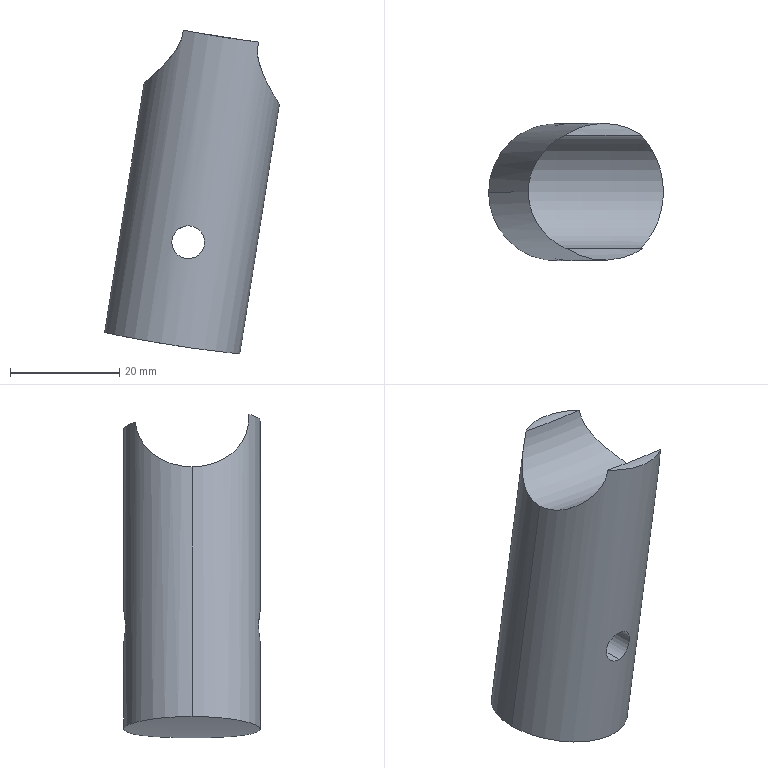Part | SolidWorks | features HoleWzd 2, RefAxis 2, 3DProfileFeature 1, CirPattern 1, ICE 1, Revolution 1 | 1 solid | 8 faces | box 31.917 x 25 x 59.146 mm | volume 23195 mm3 | cylinder 7 | torus 1 | commonest cylinder face diameters 6 x2 25 x2 352 x1 355 x1 466 x1
STEP:
#1=CARTESIAN_POINT('',(-33.477,15.509,-214.365));
#2=VERTEX_POINT('',#1);
#3=CARTESIAN_POINT('',(-33.477,15.509,-208.365));
#4=VERTEX_POINT('',#3);
#5=CARTESIAN_POINT('',(-33.477,15.509,-214.365));
#6=CARTESIAN_POINT('',(-33.869,15.494,-214.365));
#7=CARTESIAN_POINT('',(-34.266,15.498,-214.286));
#8=CARTESIAN_POINT('',(-34.808,15.531,-214.061));
#9=CARTESIAN_POINT('',(-34.984,15.546,-213.967));
#10=CARTESIAN_POINT('',(-35.311,15.582,-213.748));
#11=CARTESIAN_POINT('',(-35.461,15.603,-213.624));
#12=CARTESIAN_POINT('',(-35.738,15.648,-213.347));
#13=CARTESIAN_POINT('',(-35.864,15.672,-213.193));
#14=CARTESIAN_POINT('',(-36.08,15.719,-212.869));
#15=CARTESIAN_POINT('',(-36.172,15.743,-212.697));
#16=CARTESIAN_POINT('',(-36.324,15.786,-212.333));
#17=CARTESIAN_POINT('',(-36.381,15.805,-212.145));
#18=CARTESIAN_POINT('',(-36.457,15.836,-211.761));
#19=CARTESIAN_POINT('',(-36.477,15.849,-211.564));
#20=CARTESIAN_POINT('',(-36.477,15.864,-211.169));
#21=CARTESIAN_POINT('',(-36.458,15.867,-210.973));
#22=CARTESIAN_POINT('',(-36.381,15.863,-210.588));
#23=CARTESIAN_POINT('',(-36.323,15.856,-210.396));
#24=CARTESIAN_POINT('',(-36.172,15.834,-210.034));
#25=CARTESIAN_POINT('',(-36.08,15.819,-209.861));
#26=CARTESIAN_POINT('',(-35.861,15.782,-209.533));
#27=CARTESIAN_POINT('',(-35.735,15.76,-209.381));
#28=CARTESIAN_POINT('',(-35.459,15.715,-209.105));
#29=CARTESIAN_POINT('',(-35.307,15.691,-208.98));
#30=CARTESIAN_POINT('',(-34.98,15.643,-208.762));
#31=CARTESIAN_POINT('',(-34.808,15.62,-208.67));
#32=CARTESIAN_POINT('',(-34.448,15.578,-208.52));
#33=CARTESIAN_POINT('',(-34.257,15.559,-208.462));
#34=CARTESIAN_POINT('',(-33.872,15.528,-208.385));
#35=CARTESIAN_POINT('',(-33.676,15.516,-208.365));
#36=CARTESIAN_POINT('',(-33.477,15.509,-208.365));
#37=B_SPLINE_CURVE_WITH_KNOTS('',3,(#5,#6,#7,#8,#9,#10,#11,#12,#13,#14,#15,#16,#17,#18,#19,#20,#21,#22,#23,#24,#25,#26,#27,#28,#29,#30,#31,#32,#33,#34,#35,#36),.UNSPECIFIED.,.F.,.F.,(4,2,2,2,2,2,2,2,2,2,2,2,2,2,2,4),(0.009415,0.01059,0.01118,0.01177,0.01236,0.01294,0.01353,0.01412,0.01471,0.0153,0.01589,0.01647,0.01706,0.01765,0.01824,0.01883),.UNSPECIFIED.);
#38=EDGE_CURVE('',#2,#4,#37,.T.);
#39=ORIENTED_EDGE('',*,*,#38,.F.);
#40=CARTESIAN_POINT('',(-33.477,40.491,-214.365));
#41=VERTEX_POINT('',#40);
#42=CARTESIAN_POINT('',(-33.477,40.5,-214.365));
#43=DIRECTION('',(0.,1.,0.));
#44=VECTOR('',#43,1000.);
#45=LINE('',#42,#44);
#46=EDGE_CURVE('',#2,#41,#45,.T.);
#47=ORIENTED_EDGE('',*,*,#46,.T.);
#48=CARTESIAN_POINT('',(-33.477,40.491,-208.365));
#49=VERTEX_POINT('',#48);
#50=CARTESIAN_POINT('',(-33.477,40.491,-208.365));
#51=CARTESIAN_POINT('',(-33.676,40.484,-208.365));
#52=CARTESIAN_POINT('',(-33.871,40.472,-208.385));
#53=CARTESIAN_POINT('',(-34.255,40.441,-208.461));
#54=CARTESIAN_POINT('',(-34.445,40.422,-208.519));
#55=CARTESIAN_POINT('',(-34.808,40.38,-208.669));
#56=CARTESIAN_POINT('',(-34.979,40.357,-208.761));
#57=CARTESIAN_POINT('',(-35.305,40.31,-208.978));
#58=CARTESIAN_POINT('',(-35.458,40.285,-209.104));
#59=CARTESIAN_POINT('',(-35.735,40.24,-209.38));
#60=CARTESIAN_POINT('',(-35.859,40.218,-209.531));
#61=CARTESIAN_POINT('',(-36.078,40.181,-209.858));
#62=CARTESIAN_POINT('',(-36.172,40.166,-210.033));
#63=CARTESIAN_POINT('',(-36.322,40.144,-210.394));
#64=CARTESIAN_POINT('',(-36.38,40.137,-210.584));
#65=CARTESIAN_POINT('',(-36.458,40.133,-210.972));
#66=CARTESIAN_POINT('',(-36.477,40.136,-211.168));
#67=CARTESIAN_POINT('',(-36.477,40.151,-211.56));
#68=CARTESIAN_POINT('',(-36.457,40.163,-211.76));
#69=CARTESIAN_POINT('',(-36.381,40.195,-212.144));
#70=CARTESIAN_POINT('',(-36.324,40.214,-212.331));
#71=CARTESIAN_POINT('',(-36.174,40.257,-212.695));
#72=CARTESIAN_POINT('',(-36.08,40.281,-212.869));
#73=CARTESIAN_POINT('',(-35.864,40.328,-213.193));
#74=CARTESIAN_POINT('',(-35.74,40.352,-213.345));
#75=CARTESIAN_POINT('',(-35.461,40.397,-213.624));
#76=CARTESIAN_POINT('',(-35.31,40.418,-213.748));
#77=CARTESIAN_POINT('',(-34.986,40.454,-213.966));
#78=CARTESIAN_POINT('',(-34.81,40.469,-214.06));
#79=CARTESIAN_POINT('',(-34.446,40.491,-214.211));
#80=CARTESIAN_POINT('',(-34.259,40.497,-214.268));
#81=CARTESIAN_POINT('',(-33.873,40.501,-214.346));
#82=CARTESIAN_POINT('',(-33.673,40.498,-214.365));
#83=CARTESIAN_POINT('',(-33.477,40.491,-214.365));
#84=B_SPLINE_CURVE_WITH_KNOTS('',3,(#50,#51,#52,#53,#54,#55,#56,#57,#58,#59,#60,#61,#62,#63,#64,#65,#66,#67,#68,#69,#70,#71,#72,#73,#74,#75,#76,#77,#78,#79,#80,#81,#82,#83),.UNSPECIFIED.,.F.,.F.,(4,2,2,2,2,2,2,2,2,2,2,2,2,2,2,2,4),(0.,0.0005883,0.001177,0.001765,0.002353,0.002942,0.00353,0.004118,0.004707,0.005295,0.005883,0.006472,0.00706,0.007648,0.008236,0.008825,0.009413),.UNSPECIFIED.);
#85=EDGE_CURVE('',#49,#41,#84,.T.);
#86=ORIENTED_EDGE('',*,*,#85,.F.);
#87=CARTESIAN_POINT('',(-33.477,40.5,-208.365));
#88=DIRECTION('',(0.,1.,0.));
#89=VECTOR('',#88,1000.);
#90=LINE('',#87,#89);
#91=EDGE_CURVE('',#4,#49,#90,.T.);
#92=ORIENTED_EDGE('',*,*,#91,.F.);
#93=EDGE_LOOP('',(#39,#47,#86,#92));
#94=FACE_OUTER_BOUND('',#93,.T.);
#95=CARTESIAN_POINT('',(-33.477,40.5,-211.365));
#96=DIRECTION('',(0.,1.,0.));
#97=DIRECTION('',(0.,0.,1.));
#98=AXIS2_PLACEMENT_3D('',#95,#96,#97);
#99=CYLINDRICAL_SURFACE('',#98,3.);
#100=ADVANCED_FACE('',(#94),#99,.F.);
#101=ORIENTED_EDGE('',*,*,#85,.T.);
#102=CARTESIAN_POINT('',(-33.477,40.491,-214.365));
#103=CARTESIAN_POINT('',(-33.085,40.477,-214.365));
#104=CARTESIAN_POINT('',(-32.69,40.443,-214.286));
#105=CARTESIAN_POINT('',(-32.149,40.38,-214.062));
#106=CARTESIAN_POINT('',(-31.974,40.357,-213.969));
#107=CARTESIAN_POINT('',(-31.648,40.309,-213.751));
#108=CARTESIAN_POINT('',(-31.497,40.285,-213.628));
#109=CARTESIAN_POINT('',(-31.221,40.24,-213.352));
#110=CARTESIAN_POINT('',(-31.094,40.218,-213.198));
#111=CARTESIAN_POINT('',(-30.876,40.182,-212.873));
#112=CARTESIAN_POINT('',(-30.784,40.166,-212.701));
#113=CARTESIAN_POINT('',(-30.556,40.133,-212.154));
#114=CARTESIAN_POINT('',(-30.477,40.129,-211.762));
#115=CARTESIAN_POINT('',(-30.477,40.151,-211.169));
#116=CARTESIAN_POINT('',(-30.496,40.163,-210.974));
#117=CARTESIAN_POINT('',(-30.572,40.195,-210.589));
#118=CARTESIAN_POINT('',(-30.63,40.214,-210.398));
#119=CARTESIAN_POINT('',(-30.78,40.257,-210.037));
#120=CARTESIAN_POINT('',(-30.872,40.28,-209.865));
#121=CARTESIAN_POINT('',(-31.089,40.328,-209.538));
#122=CARTESIAN_POINT('',(-31.215,40.352,-209.385));
#123=CARTESIAN_POINT('',(-31.49,40.397,-209.11));
#124=CARTESIAN_POINT('',(-31.641,40.418,-208.984));
#125=CARTESIAN_POINT('',(-31.969,40.454,-208.764));
#126=CARTESIAN_POINT('',(-32.142,40.469,-208.672));
#127=CARTESIAN_POINT('',(-32.503,40.491,-208.521));
#128=CARTESIAN_POINT('',(-32.694,40.497,-208.462));
#129=CARTESIAN_POINT('',(-33.082,40.501,-208.385));
#130=CARTESIAN_POINT('',(-33.278,40.499,-208.365));
#131=CARTESIAN_POINT('',(-33.477,40.491,-208.365));
#132=B_SPLINE_CURVE_WITH_KNOTS('',3,(#102,#103,#104,#105,#106,#107,#108,#109,#110,#111,#112,#113,#114,#115,#116,#117,#118,#119,#120,#121,#122,#123,#124,#125,#126,#127,#128,#129,#130,#131),.UNSPECIFIED.,.F.,.F.,(4,2,2,2,2,2,2,2,2,2,2,2,2,2,4),(0.009413,0.01059,0.01118,0.01177,0.01235,0.01294,0.01412,0.01471,0.01529,0.01588,0.01647,0.01706,0.01765,0.01824,0.01882),.UNSPECIFIED.);
#133=EDGE_CURVE('',#41,#49,#132,.T.);
#134=ORIENTED_EDGE('',*,*,#133,.T.);
#135=EDGE_LOOP('',(#101,#134));
#136=FACE_BOUND('',#135,.T.);
#137=CARTESIAN_POINT('',(-48.743,28.,-227.845));
#138=VERTEX_POINT('',#137);
#139=CARTESIAN_POINT('',(-24.051,28.,-231.755));
#140=VERTEX_POINT('',#139);
#141=CARTESIAN_POINT('',(-48.743,28.,-227.845));
#142=CARTESIAN_POINT('',(-48.743,28.816,-227.845));
#143=CARTESIAN_POINT('',(-48.665,29.626,-227.861));
#144=CARTESIAN_POINT('',(-48.431,30.835,-227.911));
#145=CARTESIAN_POINT('',(-48.332,31.237,-227.932));
#146=CARTESIAN_POINT('',(-48.099,32.02,-227.981));
#147=CARTESIAN_POINT('',(-47.83,32.788,-228.038));
#148=CARTESIAN_POINT('',(-47.489,33.525,-228.109));
#149=CARTESIAN_POINT('',(-47.112,34.246,-228.187));
#150=CARTESIAN_POINT('',(-46.904,34.6,-228.23));
#151=CARTESIAN_POINT('',(-46.232,35.626,-228.368));
#152=CARTESIAN_POINT('',(-45.724,36.256,-228.47));
#153=CARTESIAN_POINT('',(-44.876,37.121,-228.638));
#154=CARTESIAN_POINT('',(-44.579,37.396,-228.696));
#155=CARTESIAN_POINT('',(-43.955,37.918,-228.817));
#156=CARTESIAN_POINT('',(-43.629,38.164,-228.879));
#157=CARTESIAN_POINT('',(-42.627,38.846,-229.069));
#158=CARTESIAN_POINT('',(-41.921,39.23,-229.199));
#159=CARTESIAN_POINT('',(-40.805,39.701,-229.399));
#160=CARTESIAN_POINT('',(-40.421,39.841,-229.467));
#161=CARTESIAN_POINT('',(-39.647,40.08,-229.602));
#162=CARTESIAN_POINT('',(-39.256,40.179,-229.67));
#163=CARTESIAN_POINT('',(-38.075,40.418,-229.869));
#164=CARTESIAN_POINT('',(-37.274,40.499,-230.001));
#165=CARTESIAN_POINT('',(-36.052,40.5,-230.194));
#166=CARTESIAN_POINT('',(-35.646,40.48,-230.258));
#167=CARTESIAN_POINT('',(-34.843,40.401,-230.38));
#168=CARTESIAN_POINT('',(-34.444,40.341,-230.44));
#169=CARTESIAN_POINT('',(-33.654,40.183,-230.557));
#170=CARTESIAN_POINT('',(-33.262,40.084,-230.614));
#171=CARTESIAN_POINT('',(-32.485,39.847,-230.725));
#172=CARTESIAN_POINT('',(-32.099,39.708,-230.779));
#173=CARTESIAN_POINT('',(-30.972,39.238,-230.934));
#174=CARTESIAN_POINT('',(-30.26,38.854,-231.028));
#175=CARTESIAN_POINT('',(-28.912,37.949,-231.2));
#176=CARTESIAN_POINT('',(-28.273,37.421,-231.279));
#177=CARTESIAN_POINT('',(-27.126,36.269,-231.416));
#178=CARTESIAN_POINT('',(-26.611,35.64,-231.476));
#179=CARTESIAN_POINT('',(-25.929,34.617,-231.553));
#180=CARTESIAN_POINT('',(-25.717,34.262,-231.576));
#181=CARTESIAN_POINT('',(-25.333,33.54,-231.619));
#182=CARTESIAN_POINT('',(-24.985,32.804,-231.657));
#183=CARTESIAN_POINT('',(-24.711,32.037,-231.686));
#184=CARTESIAN_POINT('',(-24.473,31.255,-231.711));
#185=CARTESIAN_POINT('',(-24.373,30.856,-231.722));
#186=CARTESIAN_POINT('',(-24.131,29.643,-231.747));
#187=CARTESIAN_POINT('',(-24.051,28.826,-231.755));
#188=CARTESIAN_POINT('',(-24.051,28.,-231.755));
#189=B_SPLINE_CURVE_WITH_KNOTS('',3,(#141,#142,#143,#144,#145,#146,#147,#148,#149,#150,#151,#152,#153,#154,#155,#156,#157,#158,#159,#160,#161,#162,#163,#164,#165,#166,#167,#168,#169,#170,#171,#172,#173,#174,#175,#176,#177,#178,#179,#180,#181,#182,#183,#184,#185,#186,#187,#188),.UNSPECIFIED.,.F.,.F.,(4,2,2,1,2,2,2,2,2,2,2,2,2,2,2,2,2,2,2,2,2,1,2,2,4),(0.03909,0.04153,0.04275,0.04397,0.04519,0.04641,0.04886,0.05008,0.0513,0.05374,0.05496,0.05618,0.05863,0.05985,0.06107,0.06229,0.06351,0.06595,0.0684,0.07084,0.07206,0.07328,0.0745,0.07572,0.07817),.UNSPECIFIED.);
#190=EDGE_CURVE('',#138,#140,#189,.T.);
#191=ORIENTED_EDGE('',*,*,#190,.F.);
#192=CARTESIAN_POINT('',(-41.518,28.,-182.23));
#193=VERTEX_POINT('',#192);
#194=CARTESIAN_POINT('',(-54.048,28.,-261.343));
#195=DIRECTION('',(0.1564,0.,0.9877));
#196=VECTOR('',#195,1000.);
#197=LINE('',#194,#196);
#198=EDGE_CURVE('',#138,#193,#197,.T.);
#199=ORIENTED_EDGE('',*,*,#198,.T.);
#200=CARTESIAN_POINT('',(-34.666,38.352,-174.082));
#201=VERTEX_POINT('',#200);
#202=CARTESIAN_POINT('',(-34.666,38.352,-174.082));
#203=CARTESIAN_POINT('',(-34.868,38.286,-174.737));
#204=CARTESIAN_POINT('',(-35.153,38.157,-175.336));
#205=CARTESIAN_POINT('',(-35.654,37.884,-176.181));
#206=CARTESIAN_POINT('',(-35.834,37.778,-176.454));
#207=CARTESIAN_POINT('',(-36.204,37.545,-176.976));
#208=CARTESIAN_POINT('',(-36.394,37.418,-177.225));
#209=CARTESIAN_POINT('',(-36.975,37.002,-177.944));
#210=CARTESIAN_POINT('',(-37.373,36.681,-178.387));
#211=CARTESIAN_POINT('',(-37.968,36.131,-179.01));
#212=CARTESIAN_POINT('',(-38.166,35.936,-179.21));
#213=CARTESIAN_POINT('',(-38.551,35.529,-179.591));
#214=CARTESIAN_POINT('',(-38.739,35.315,-179.772));
#215=CARTESIAN_POINT('',(-39.29,34.644,-180.293));
#216=CARTESIAN_POINT('',(-39.636,34.157,-180.608));
#217=CARTESIAN_POINT('',(-40.272,33.086,-181.172));
#218=CARTESIAN_POINT('',(-40.552,32.516,-181.414));
#219=CARTESIAN_POINT('',(-40.901,31.612,-181.712));
#220=CARTESIAN_POINT('',(-41.005,31.301,-181.801));
#221=CARTESIAN_POINT('',(-41.189,30.662,-181.955));
#222=CARTESIAN_POINT('',(-41.267,30.335,-182.021));
#223=CARTESIAN_POINT('',(-41.454,29.349,-182.177));
#224=CARTESIAN_POINT('',(-41.518,28.681,-182.23));
#225=CARTESIAN_POINT('',(-41.518,28.,-182.23));
#226=B_SPLINE_CURVE_WITH_KNOTS('',3,(#202,#203,#204,#205,#206,#207,#208,#209,#210,#211,#212,#213,#214,#215,#216,#217,#218,#219,#220,#221,#222,#223,#224,#225),.UNSPECIFIED.,.F.,.F.,(4,2,2,2,2,2,2,2,2,2,2,4),(0.000002056,0.00203,0.003044,0.004059,0.006087,0.007101,0.008115,0.01014,0.01217,0.01319,0.0142,0.01623),.UNSPECIFIED.);
#227=EDGE_CURVE('',#201,#193,#226,.T.);
#228=ORIENTED_EDGE('',*,*,#227,.F.);
#229=CARTESIAN_POINT('',(-20.825,38.352,-176.274));
#230=VERTEX_POINT('',#229);
#231=CARTESIAN_POINT('',(-20.825,38.352,-176.274));
#232=CARTESIAN_POINT('',(-21.854,39.052,-176.153));
#233=CARTESIAN_POINT('',(-22.958,39.584,-176.013));
#234=CARTESIAN_POINT('',(-24.429,40.04,-175.811));
#235=CARTESIAN_POINT('',(-24.729,40.121,-175.769));
#236=CARTESIAN_POINT('',(-25.33,40.258,-175.684));
#237=CARTESIAN_POINT('',(-25.631,40.316,-175.64));
#238=CARTESIAN_POINT('',(-26.537,40.453,-175.506));
#239=CARTESIAN_POINT('',(-27.145,40.499,-175.413));
#240=CARTESIAN_POINT('',(-28.367,40.501,-175.22));
#241=CARTESIAN_POINT('',(-28.986,40.454,-175.118));
#242=CARTESIAN_POINT('',(-30.194,40.271,-174.914));
#243=CARTESIAN_POINT('',(-30.787,40.135,-174.811));
#244=CARTESIAN_POINT('',(-31.658,39.865,-174.654));
#245=CARTESIAN_POINT('',(-31.946,39.764,-174.602));
#246=CARTESIAN_POINT('',(-32.515,39.539,-174.497));
#247=CARTESIAN_POINT('',(-32.797,39.414,-174.444));
#248=CARTESIAN_POINT('',(-33.627,39.011,-174.286));
#249=CARTESIAN_POINT('',(-34.158,38.702,-174.183));
#250=CARTESIAN_POINT('',(-34.666,38.352,-174.082));
#251=B_SPLINE_CURVE_WITH_KNOTS('',3,(#231,#232,#233,#234,#235,#236,#237,#238,#239,#240,#241,#242,#243,#244,#245,#246,#247,#248,#249,#250),.UNSPECIFIED.,.F.,.F.,(4,2,2,2,2,2,2,2,2,4),(0.,0.003698,0.004623,0.005547,0.007396,0.009246,0.01109,0.01202,0.01294,0.01479),.UNSPECIFIED.);
#252=EDGE_CURVE('',#230,#201,#251,.T.);
#253=ORIENTED_EDGE('',*,*,#252,.F.);
#254=CARTESIAN_POINT('',(-16.826,28.,-186.141));
#255=VERTEX_POINT('',#254);
#256=CARTESIAN_POINT('',(-16.826,28.,-186.141));
#257=CARTESIAN_POINT('',(-16.826,28.337,-186.141));
#258=CARTESIAN_POINT('',(-16.837,28.675,-186.124));
#259=CARTESIAN_POINT('',(-16.882,29.352,-186.053));
#260=CARTESIAN_POINT('',(-16.915,29.688,-186.));
#261=CARTESIAN_POINT('',(-17.045,30.673,-185.793));
#262=CARTESIAN_POINT('',(-17.172,31.308,-185.589));
#263=CARTESIAN_POINT('',(-17.496,32.525,-185.062));
#264=CARTESIAN_POINT('',(-17.687,33.092,-184.746));
#265=CARTESIAN_POINT('',(-18.007,33.888,-184.201));
#266=CARTESIAN_POINT('',(-18.119,34.145,-184.006));
#267=CARTESIAN_POINT('',(-18.351,34.638,-183.597));
#268=CARTESIAN_POINT('',(-18.47,34.873,-183.384));
#269=CARTESIAN_POINT('',(-18.834,35.545,-182.716));
#270=CARTESIAN_POINT('',(-19.085,35.95,-182.236));
#271=CARTESIAN_POINT('',(-19.458,36.5,-181.46));
#272=CARTESIAN_POINT('',(-19.581,36.672,-181.193));
#273=CARTESIAN_POINT('',(-19.819,36.993,-180.648));
#274=CARTESIAN_POINT('',(-19.934,37.142,-180.369));
#275=CARTESIAN_POINT('',(-20.262,37.556,-179.51));
#276=CARTESIAN_POINT('',(-20.458,37.788,-178.909));
#277=CARTESIAN_POINT('',(-20.675,38.063,-177.949));
#278=CARTESIAN_POINT('',(-20.734,38.142,-177.619));
#279=CARTESIAN_POINT('',(-20.811,38.27,-176.953));
#280=CARTESIAN_POINT('',(-20.83,38.319,-176.616));
#281=CARTESIAN_POINT('',(-20.825,38.352,-176.274));
#282=B_SPLINE_CURVE_WITH_KNOTS('',3,(#256,#257,#258,#259,#260,#261,#262,#263,#264,#265,#266,#267,#268,#269,#270,#271,#272,#273,#274,#275,#276,#277,#278,#279,#280,#281),.UNSPECIFIED.,.F.,.F.,(4,2,2,2,2,2,2,2,2,2,2,2,4),(0.05114,0.05215,0.05315,0.05516,0.05717,0.05818,0.05918,0.06119,0.0622,0.0632,0.06521,0.06622,0.06722),.UNSPECIFIED.);
#283=EDGE_CURVE('',#255,#230,#282,.T.);
#284=ORIENTED_EDGE('',*,*,#283,.F.);
#285=CARTESIAN_POINT('',(-29.356,28.,-265.254));
#286=DIRECTION('',(0.1564,0.,0.9877));
#287=VECTOR('',#286,1000.);
#288=LINE('',#285,#287);
#289=EDGE_CURVE('',#140,#255,#288,.T.);
#290=ORIENTED_EDGE('',*,*,#289,.F.);
#291=EDGE_LOOP('',(#191,#199,#228,#253,#284,#290));
#292=FACE_OUTER_BOUND('',#291,.T.);
#293=CARTESIAN_POINT('',(-41.702,28.,-263.299));
#294=DIRECTION('',(0.1564,0.,0.9877));
#295=DIRECTION('',(0.9877,0.,-0.1564));
#296=AXIS2_PLACEMENT_3D('',#293,#294,#295);
#297=CYLINDRICAL_SURFACE('',#296,12.5);
#298=ADVANCED_FACE('',(#136,#292),#297,.T.);
#299=CARTESIAN_POINT('',(-24.051,28.,-231.755));
#300=CARTESIAN_POINT('',(-24.051,27.174,-231.755));
#301=CARTESIAN_POINT('',(-24.131,26.362,-231.747));
#302=CARTESIAN_POINT('',(-24.369,25.163,-231.722));
#303=CARTESIAN_POINT('',(-24.467,24.767,-231.712));
#304=CARTESIAN_POINT('',(-24.704,23.982,-231.687));
#305=CARTESIAN_POINT('',(-24.843,23.591,-231.672));
#306=CARTESIAN_POINT('',(-25.312,22.456,-231.621));
#307=CARTESIAN_POINT('',(-25.694,21.738,-231.579));
#308=CARTESIAN_POINT('',(-26.371,20.719,-231.503));
#309=CARTESIAN_POINT('',(-26.615,20.388,-231.475));
#310=CARTESIAN_POINT('',(-27.135,19.751,-231.415));
#311=CARTESIAN_POINT('',(-27.408,19.448,-231.383));
#312=CARTESIAN_POINT('',(-28.268,18.583,-231.28));
#313=CARTESIAN_POINT('',(-28.893,18.066,-231.203));
#314=CARTESIAN_POINT('',(-29.91,17.38,-231.073));
#315=CARTESIAN_POINT('',(-30.262,17.168,-231.027));
#316=CARTESIAN_POINT('',(-30.977,16.782,-230.932));
#317=CARTESIAN_POINT('',(-31.708,16.434,-230.833));
#318=CARTESIAN_POINT('',(-32.468,16.159,-230.727));
#319=CARTESIAN_POINT('',(-33.243,15.921,-230.617));
#320=CARTESIAN_POINT('',(-33.64,15.82,-230.559));
#321=CARTESIAN_POINT('',(-34.837,15.58,-230.382));
#322=CARTESIAN_POINT('',(-35.639,15.5,-230.26));
#323=CARTESIAN_POINT('',(-36.848,15.5,-230.068));
#324=CARTESIAN_POINT('',(-37.251,15.52,-230.003));
#325=CARTESIAN_POINT('',(-38.06,15.6,-229.871));
#326=CARTESIAN_POINT('',(-38.463,15.661,-229.804));
#327=CARTESIAN_POINT('',(-39.649,15.9,-229.603));
#328=CARTESIAN_POINT('',(-40.416,16.136,-229.469));
#329=CARTESIAN_POINT('',(-41.534,16.606,-229.269));
#330=CARTESIAN_POINT('',(-41.903,16.783,-229.201));
#331=CARTESIAN_POINT('',(-42.615,17.17,-229.07));
#332=CARTESIAN_POINT('',(-42.959,17.38,-229.006));
#333=CARTESIAN_POINT('',(-43.958,18.059,-228.817));
#334=CARTESIAN_POINT('',(-44.578,18.576,-228.697));
#335=CARTESIAN_POINT('',(-45.724,19.743,-228.47));
#336=CARTESIAN_POINT('',(-46.232,20.375,-228.368));
#337=CARTESIAN_POINT('',(-46.898,21.39,-228.232));
#338=CARTESIAN_POINT('',(-47.104,21.74,-228.189));
#339=CARTESIAN_POINT('',(-47.483,22.463,-228.11));
#340=CARTESIAN_POINT('',(-47.657,22.838,-228.074));
#341=CARTESIAN_POINT('',(-48.118,23.974,-227.977));
#342=CARTESIAN_POINT('',(-48.35,24.753,-227.928));
#343=CARTESIAN_POINT('',(-48.585,25.955,-227.878));
#344=CARTESIAN_POINT('',(-48.644,26.362,-227.866));
#345=CARTESIAN_POINT('',(-48.723,27.183,-227.849));
#346=CARTESIAN_POINT('',(-48.743,27.592,-227.845));
#347=CARTESIAN_POINT('',(-48.743,28.,-227.845));
#348=B_SPLINE_CURVE_WITH_KNOTS('',3,(#299,#300,#301,#302,#303,#304,#305,#306,#307,#308,#309,#310,#311,#312,#313,#314,#315,#316,#317,#318,#319,#320,#321,#322,#323,#324,#325,#326,#327,#328,#329,#330,#331,#332,#333,#334,#335,#336,#337,#338,#339,#340,#341,#342,#343,#344,#345,#346,#347),.UNSPECIFIED.,.F.,.F.,(4,2,2,2,2,2,2,2,2,1,2,2,2,2,2,2,2,2,2,2,2,2,2,2,4),(0.,0.002443,0.003664,0.004886,0.007329,0.00855,0.009772,0.01221,0.01344,0.01466,0.01588,0.0171,0.01954,0.02077,0.02199,0.02443,0.02565,0.02687,0.02932,0.03176,0.03298,0.0342,0.03664,0.03787,0.03909),.UNSPECIFIED.);
#349=EDGE_CURVE('',#140,#138,#348,.T.);
#350=ORIENTED_EDGE('',*,*,#349,.T.);
#351=ORIENTED_EDGE('',*,*,#190,.T.);
#352=EDGE_LOOP('',(#350,#351));
#353=FACE_OUTER_BOUND('',#352,.T.);
#354=CARTESIAN_POINT('',(0.,33.104,0.));
#355=DIRECTION('',(0.,-1.,0.));
#356=DIRECTION('',(0.,0.,-1.));
#357=AXIS2_PLACEMENT_3D('',#354,#355,#356);
#358=CYLINDRICAL_SURFACE('',#357,233.);
#359=ADVANCED_FACE('',(#353),#358,.T.);
#360=ORIENTED_EDGE('',*,*,#198,.F.);
#361=ORIENTED_EDGE('',*,*,#349,.F.);
#362=ORIENTED_EDGE('',*,*,#289,.T.);
#363=CARTESIAN_POINT('',(-20.644,17.612,-174.785));
#364=VERTEX_POINT('',#363);
#365=CARTESIAN_POINT('',(-20.644,17.612,-174.785));
#366=CARTESIAN_POINT('',(-20.729,17.594,-175.149));
#367=CARTESIAN_POINT('',(-20.783,17.596,-175.516));
#368=CARTESIAN_POINT('',(-20.835,17.64,-176.251));
#369=CARTESIAN_POINT('',(-20.831,17.681,-176.623));
#370=CARTESIAN_POINT('',(-20.743,17.862,-177.727));
#371=CARTESIAN_POINT('',(-20.587,18.051,-178.425));
#372=CARTESIAN_POINT('',(-20.281,18.425,-179.433));
#373=CARTESIAN_POINT('',(-20.166,18.565,-179.76));
#374=CARTESIAN_POINT('',(-19.926,18.868,-180.391));
#375=CARTESIAN_POINT('',(-19.799,19.032,-180.696));
#376=CARTESIAN_POINT('',(-19.538,19.386,-181.287));
#377=CARTESIAN_POINT('',(-19.404,19.576,-181.574));
#378=CARTESIAN_POINT('',(-19.133,19.982,-182.13));
#379=CARTESIAN_POINT('',(-18.996,20.199,-182.4));
#380=CARTESIAN_POINT('',(-18.588,20.889,-183.178));
#381=CARTESIAN_POINT('',(-18.325,21.392,-183.648));
#382=CARTESIAN_POINT('',(-17.961,22.219,-184.279));
#383=CARTESIAN_POINT('',(-17.845,22.507,-184.477));
#384=CARTESIAN_POINT('',(-17.625,23.111,-184.847));
#385=CARTESIAN_POINT('',(-17.52,23.428,-185.02));
#386=CARTESIAN_POINT('',(-17.238,24.401,-185.484));
#387=CARTESIAN_POINT('',(-17.087,25.083,-185.725));
#388=CARTESIAN_POINT('',(-16.932,26.162,-185.974));
#389=CARTESIAN_POINT('',(-16.892,26.53,-186.037));
#390=CARTESIAN_POINT('',(-16.839,27.263,-186.12));
#391=CARTESIAN_POINT('',(-16.826,27.631,-186.141));
#392=CARTESIAN_POINT('',(-16.826,28.,-186.141));
#393=B_SPLINE_CURVE_WITH_KNOTS('',3,(#365,#366,#367,#368,#369,#370,#371,#372,#373,#374,#375,#376,#377,#378,#379,#380,#381,#382,#383,#384,#385,#386,#387,#388,#389,#390,#391,#392),.UNSPECIFIED.,.F.,.F.,(4,2,2,2,2,2,2,2,2,2,2,2,2,4),(0.03353,0.03463,0.03573,0.03793,0.03903,0.04013,0.04124,0.04234,0.04454,0.04564,0.04674,0.04894,0.05004,0.05114),.UNSPECIFIED.);
#394=EDGE_CURVE('',#364,#255,#393,.T.);
#395=ORIENTED_EDGE('',*,*,#394,.F.);
#396=CARTESIAN_POINT('',(-34.378,17.612,-172.61));
#397=VERTEX_POINT('',#396);
#398=CARTESIAN_POINT('',(-34.378,17.612,-172.61));
#399=CARTESIAN_POINT('',(-33.368,16.923,-172.811));
#400=CARTESIAN_POINT('',(-32.282,16.401,-173.018));
#401=CARTESIAN_POINT('',(-30.832,15.952,-173.279));
#402=CARTESIAN_POINT('',(-30.536,15.873,-173.331));
#403=CARTESIAN_POINT('',(-29.944,15.737,-173.434));
#404=CARTESIAN_POINT('',(-29.646,15.681,-173.485));
#405=CARTESIAN_POINT('',(-28.751,15.546,-173.637));
#406=CARTESIAN_POINT('',(-28.149,15.501,-173.735));
#407=CARTESIAN_POINT('',(-26.938,15.499,-173.927));
#408=CARTESIAN_POINT('',(-26.324,15.545,-174.021));
#409=CARTESIAN_POINT('',(-25.121,15.725,-174.199));
#410=CARTESIAN_POINT('',(-24.53,15.859,-174.283));
#411=CARTESIAN_POINT('',(-23.371,16.213,-174.442));
#412=CARTESIAN_POINT('',(-22.799,16.434,-174.518));
#413=CARTESIAN_POINT('',(-21.689,16.963,-174.659));
#414=CARTESIAN_POINT('',(-21.156,17.267,-174.725));
#415=CARTESIAN_POINT('',(-20.644,17.612,-174.785));
#416=B_SPLINE_CURVE_WITH_KNOTS('',3,(#398,#399,#400,#401,#402,#403,#404,#405,#406,#407,#408,#409,#410,#411,#412,#413,#414,#415),.UNSPECIFIED.,.F.,.F.,(4,2,2,2,2,2,2,2,4),(0.,0.003666,0.004583,0.005499,0.007332,0.009165,0.011,0.01283,0.01466),.UNSPECIFIED.);
#417=EDGE_CURVE('',#397,#364,#416,.T.);
#418=ORIENTED_EDGE('',*,*,#417,.F.);
#419=CARTESIAN_POINT('',(-41.518,28.,-182.23));
#420=CARTESIAN_POINT('',(-41.518,27.629,-182.23));
#421=CARTESIAN_POINT('',(-41.499,27.254,-182.214));
#422=CARTESIAN_POINT('',(-41.422,26.521,-182.15));
#423=CARTESIAN_POINT('',(-41.366,26.16,-182.103));
#424=CARTESIAN_POINT('',(-41.217,25.447,-181.979));
#425=CARTESIAN_POINT('',(-41.125,25.095,-181.902));
#426=CARTESIAN_POINT('',(-40.908,24.405,-181.718));
#427=CARTESIAN_POINT('',(-40.784,24.072,-181.613));
#428=CARTESIAN_POINT('',(-40.511,23.427,-181.378));
#429=CARTESIAN_POINT('',(-40.361,23.115,-181.248));
#430=CARTESIAN_POINT('',(-40.037,22.511,-180.964));
#431=CARTESIAN_POINT('',(-39.863,22.218,-180.809));
#432=CARTESIAN_POINT('',(-39.316,21.383,-180.317));
#433=CARTESIAN_POINT('',(-38.919,20.88,-179.949));
#434=CARTESIAN_POINT('',(-38.293,20.193,-179.337));
#435=CARTESIAN_POINT('',(-38.078,19.976,-179.122));
#436=CARTESIAN_POINT('',(-37.648,19.569,-178.676));
#437=CARTESIAN_POINT('',(-37.431,19.38,-178.444));
#438=CARTESIAN_POINT('',(-36.786,18.85,-177.721));
#439=CARTESIAN_POINT('',(-36.358,18.548,-177.202));
#440=CARTESIAN_POINT('',(-35.554,18.049,-176.048));
#441=CARTESIAN_POINT('',(-35.189,17.86,-175.429));
#442=CARTESIAN_POINT('',(-34.836,17.71,-174.579));
#443=CARTESIAN_POINT('',(-34.771,17.685,-174.404));
#444=CARTESIAN_POINT('',(-34.655,17.644,-174.054));
#445=CARTESIAN_POINT('',(-34.603,17.628,-173.877));
#446=CARTESIAN_POINT('',(-34.47,17.596,-173.343));
#447=CARTESIAN_POINT('',(-34.41,17.594,-172.98));
#448=CARTESIAN_POINT('',(-34.378,17.612,-172.61));
#449=B_SPLINE_CURVE_WITH_KNOTS('',3,(#419,#420,#421,#422,#423,#424,#425,#426,#427,#428,#429,#430,#431,#432,#433,#434,#435,#436,#437,#438,#439,#440,#441,#442,#443,#444,#445,#446,#447,#448),.UNSPECIFIED.,.F.,.F.,(4,2,2,2,2,2,2,2,2,2,2,2,2,2,4),(0.01623,0.01733,0.01844,0.01954,0.02065,0.02176,0.02286,0.02507,0.02618,0.02728,0.02949,0.0317,0.03226,0.03281,0.03391),.UNSPECIFIED.);
#450=EDGE_CURVE('',#193,#397,#449,.T.);
#451=ORIENTED_EDGE('',*,*,#450,.F.);
#452=EDGE_LOOP('',(#360,#361,#362,#395,#418,#451));
#453=FACE_OUTER_BOUND('',#452,.T.);
#454=CARTESIAN_POINT('',(-33.477,15.509,-208.365));
#455=CARTESIAN_POINT('',(-33.278,15.501,-208.365));
#456=CARTESIAN_POINT('',(-33.083,15.499,-208.385));
#457=CARTESIAN_POINT('',(-32.698,15.502,-208.462));
#458=CARTESIAN_POINT('',(-32.506,15.509,-208.52));
#459=CARTESIAN_POINT('',(-32.143,15.531,-208.671));
#460=CARTESIAN_POINT('',(-31.97,15.546,-208.764));
#461=CARTESIAN_POINT('',(-31.644,15.582,-208.982));
#462=CARTESIAN_POINT('',(-31.49,15.603,-209.109));
#463=CARTESIAN_POINT('',(-31.077,15.67,-209.523));
#464=CARTESIAN_POINT('',(-30.855,15.722,-209.857));
#465=CARTESIAN_POINT('',(-30.631,15.786,-210.397));
#466=CARTESIAN_POINT('',(-30.573,15.805,-210.587));
#467=CARTESIAN_POINT('',(-30.496,15.837,-210.973));
#468=CARTESIAN_POINT('',(-30.477,15.849,-211.168));
#469=CARTESIAN_POINT('',(-30.477,15.864,-211.561));
#470=CARTESIAN_POINT('',(-30.497,15.867,-211.76));
#471=CARTESIAN_POINT('',(-30.574,15.863,-212.146));
#472=CARTESIAN_POINT('',(-30.631,15.856,-212.333));
#473=CARTESIAN_POINT('',(-30.858,15.823,-212.881));
#474=CARTESIAN_POINT('',(-31.08,15.783,-213.212));
#475=CARTESIAN_POINT('',(-31.498,15.715,-213.628));
#476=CARTESIAN_POINT('',(-31.648,15.691,-213.752));
#477=CARTESIAN_POINT('',(-31.973,15.643,-213.968));
#478=CARTESIAN_POINT('',(-32.149,15.62,-214.062));
#479=CARTESIAN_POINT('',(-32.51,15.578,-214.212));
#480=CARTESIAN_POINT('',(-32.697,15.559,-214.269));
#481=CARTESIAN_POINT('',(-33.082,15.528,-214.346));
#482=CARTESIAN_POINT('',(-33.281,15.516,-214.365));
#483=CARTESIAN_POINT('',(-33.477,15.509,-214.365));
#484=B_SPLINE_CURVE_WITH_KNOTS('',3,(#454,#455,#456,#457,#458,#459,#460,#461,#462,#463,#464,#465,#466,#467,#468,#469,#470,#471,#472,#473,#474,#475,#476,#477,#478,#479,#480,#481,#482,#483),.UNSPECIFIED.,.F.,.F.,(4,2,2,2,2,2,2,2,2,2,2,2,2,2,4),(0.,0.0005884,0.001177,0.001765,0.002354,0.003531,0.004119,0.004707,0.005296,0.005884,0.007061,0.007649,0.008238,0.008826,0.009415),.UNSPECIFIED.);
#485=EDGE_CURVE('',#4,#2,#484,.T.);
#486=ORIENTED_EDGE('',*,*,#485,.T.);
#487=ORIENTED_EDGE('',*,*,#38,.T.);
#488=EDGE_LOOP('',(#486,#487));
#489=FACE_BOUND('',#488,.T.);
#490=CARTESIAN_POINT('',(-41.702,28.,-263.299));
#491=DIRECTION('',(0.1564,0.,0.9877));
#492=DIRECTION('',(0.9877,0.,-0.1564));
#493=AXIS2_PLACEMENT_3D('',#490,#491,#492);
#494=CYLINDRICAL_SURFACE('',#493,12.5);
#495=ADVANCED_FACE('',(#453,#489),#494,.T.);
#496=CARTESIAN_POINT('',(0.,38.352,0.));
#497=DIRECTION('',(0.,-1.,0.));
#498=DIRECTION('',(0.,0.,-1.));
#499=AXIS2_PLACEMENT_3D('',#496,#497,#498);
#500=CIRCLE('',#499,177.5);
#501=EDGE_CURVE('',#201,#230,#500,.T.);
#502=ORIENTED_EDGE('',*,*,#501,.T.);
#503=ORIENTED_EDGE('',*,*,#252,.T.);
#504=EDGE_LOOP('',(#502,#503));
#505=FACE_OUTER_BOUND('',#504,.T.);
#506=CARTESIAN_POINT('',(0.,33.104,0.));
#507=DIRECTION('',(0.,-1.,0.));
#508=DIRECTION('',(0.,0.,-1.));
#509=AXIS2_PLACEMENT_3D('',#506,#507,#508);
#510=CYLINDRICAL_SURFACE('',#509,177.5);
#511=ADVANCED_FACE('',(#505),#510,.F.);
#512=CARTESIAN_POINT('',(0.,17.612,0.));
#513=DIRECTION('',(0.,-1.,0.));
#514=DIRECTION('',(0.,0.,-1.));
#515=AXIS2_PLACEMENT_3D('',#512,#513,#514);
#516=CIRCLE('',#515,176.);
#517=EDGE_CURVE('',#397,#364,#516,.T.);
#518=ORIENTED_EDGE('',*,*,#517,.T.);
#519=ORIENTED_EDGE('',*,*,#394,.T.);
#520=ORIENTED_EDGE('',*,*,#283,.T.);
#521=ORIENTED_EDGE('',*,*,#501,.F.);
#522=ORIENTED_EDGE('',*,*,#227,.T.);
#523=ORIENTED_EDGE('',*,*,#450,.T.);
#524=EDGE_LOOP('',(#518,#519,#520,#521,#522,#523));
#525=FACE_OUTER_BOUND('',#524,.T.);
#526=CARTESIAN_POINT('',(0.,28.,0.));
#527=DIRECTION('',(0.,-1.,0.));
#528=DIRECTION('',(0.,0.,-1.));
#529=AXIS2_PLACEMENT_3D('',#526,#527,#528);
#530=TOROIDAL_SURFACE('',#529,176.5,10.4);
#531=ADVANCED_FACE('',(#525),#530,.F.);
#532=ORIENTED_EDGE('',*,*,#517,.F.);
#533=ORIENTED_EDGE('',*,*,#417,.T.);
#534=EDGE_LOOP('',(#532,#533));
#535=FACE_OUTER_BOUND('',#534,.T.);
#536=CARTESIAN_POINT('',(0.,33.104,0.));
#537=DIRECTION('',(0.,-1.,0.));
#538=DIRECTION('',(0.,0.,-1.));
#539=AXIS2_PLACEMENT_3D('',#536,#537,#538);
#540=CYLINDRICAL_SURFACE('',#539,176.);
#541=ADVANCED_FACE('',(#535),#540,.F.);
#542=ORIENTED_EDGE('',*,*,#46,.F.);
#543=ORIENTED_EDGE('',*,*,#485,.F.);
#544=ORIENTED_EDGE('',*,*,#91,.T.);
#545=ORIENTED_EDGE('',*,*,#133,.F.);
#546=EDGE_LOOP('',(#542,#543,#544,#545));
#547=FACE_OUTER_BOUND('',#546,.T.);
#548=CARTESIAN_POINT('',(-33.477,40.5,-211.365));
#549=DIRECTION('',(0.,1.,0.));
#550=DIRECTION('',(0.,0.,1.));
#551=AXIS2_PLACEMENT_3D('',#548,#549,#550);
#552=CYLINDRICAL_SURFACE('',#551,3.);
#553=ADVANCED_FACE('',(#547),#552,.F.);
#554=CLOSED_SHELL('',(#100,#298,#359,#495,#511,#531,#541,#553));
#555=MANIFOLD_SOLID_BREP('',#554);
#556=CARTESIAN_POINT('',(0.,0.,0.));
#557=DIRECTION('',(0.,0.,1.));
#558=DIRECTION('',(1.,0.,0.));
#559=AXIS2_PLACEMENT_3D('',#556,#557,#558);
#560=(LENGTH_UNIT()NAMED_UNIT(*)SI_UNIT(.MILLI.,.METRE.));
#561=UNCERTAINTY_MEASURE_WITH_UNIT(LENGTH_MEASURE(0.00001),#560,'','');
#562=(NAMED_UNIT(*)PLANE_ANGLE_UNIT()SI_UNIT($,.RADIAN.));
#563=(NAMED_UNIT(*)SI_UNIT($,.STERADIAN.)SOLID_ANGLE_UNIT());
#564=(GEOMETRIC_REPRESENTATION_CONTEXT(3)GLOBAL_UNCERTAINTY_ASSIGNED_CONTEXT((#561))GLOBAL_UNIT_ASSIGNED_CONTEXT((#560,#562,#563))REPRESENTATION_CONTEXT('',''));
#565=ADVANCED_BREP_SHAPE_REPRESENTATION('',(#555,#559),#564);